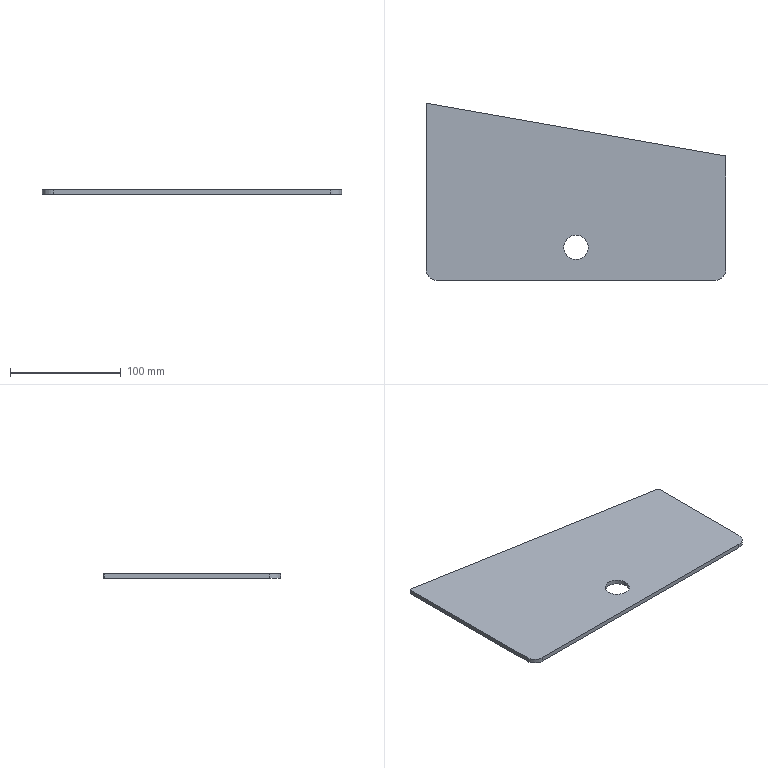Part | STEP file | 001-011-Blanking flip adjusting plate | 1 solid | 12 faces | box 270 x 159.808 x 4 mm | volume 145397 mm3 | cylinder 6 | plane 6 | commonest cylinder face diameters 2 x2 20 x2 22 x2
STEP:
#1=CARTESIAN_POINT('',(0.,0.,0.));
#2=DIRECTION('',(0.,0.,1.));
#3=DIRECTION('',(1.,0.,0.));
#4=AXIS2_PLACEMENT_3D('',#1,#2,#3);
#5=CARTESIAN_POINT('',(-11.,-50.,0.));
#6=VERTEX_POINT('',#5);
#7=CARTESIAN_POINT('',(-11.,-50.,-4.));
#8=VERTEX_POINT('',#7);
#9=CARTESIAN_POINT('',(-11.,-50.,-4.));
#10=DIRECTION('',(0.,0.,-1.));
#11=VECTOR('',#10,1.);
#12=LINE('',#9,#11);
#13=CARTESIAN_POINT('',(0.,-50.,-4.));
#14=DIRECTION('',(0.,0.,-1.));
#15=DIRECTION('',(-1.,0.,0.));
#16=AXIS2_PLACEMENT_3D('',#13,#14,#15);
#17=CYLINDRICAL_SURFACE('',#16,11.);
#18=CARTESIAN_POINT('',(6.283,0.));
#19=DIRECTION('',(0.,1.));
#20=VECTOR('',#19,1.);
#21=LINE('',#18,#20);
#22=(GEOMETRIC_REPRESENTATION_CONTEXT(2)PARAMETRIC_REPRESENTATION_CONTEXT()REPRESENTATION_CONTEXT('',''));
#23=DEFINITIONAL_REPRESENTATION('',(#21),#22);
#24=PCURVE('',#17,#23);
#25=CARTESIAN_POINT('',(0.,-50.,-4.));
#26=DIRECTION('',(0.,0.,-1.));
#27=DIRECTION('',(-1.,0.,0.));
#28=AXIS2_PLACEMENT_3D('',#25,#26,#27);
#29=CYLINDRICAL_SURFACE('',#28,11.);
#30=CARTESIAN_POINT('',(0.,0.));
#31=DIRECTION('',(0.,1.));
#32=VECTOR('',#31,1.);
#33=LINE('',#30,#32);
#34=(GEOMETRIC_REPRESENTATION_CONTEXT(2)PARAMETRIC_REPRESENTATION_CONTEXT()REPRESENTATION_CONTEXT('',''));
#35=DEFINITIONAL_REPRESENTATION('',(#33),#34);
#36=PCURVE('',#29,#35);
#37=SURFACE_CURVE('',#12,(#24,#36),.PCURVE_S1.);
#38=EDGE_CURVE('',#6,#8,#37,.T.);
#39=ORIENTED_EDGE('',*,*,#38,.T.);
#40=CARTESIAN_POINT('',(11.,-50.,-4.));
#41=VERTEX_POINT('',#40);
#42=CARTESIAN_POINT('',(0.,-50.,-4.));
#43=DIRECTION('',(0.,0.,-1.));
#44=DIRECTION('',(-1.,0.,0.));
#45=AXIS2_PLACEMENT_3D('',#42,#43,#44);
#46=CIRCLE('',#45,11.);
#47=CARTESIAN_POINT('',(0.,0.));
#48=DIRECTION('',(1.,0.));
#49=VECTOR('',#48,1.);
#50=LINE('',#47,#49);
#51=(GEOMETRIC_REPRESENTATION_CONTEXT(2)PARAMETRIC_REPRESENTATION_CONTEXT()REPRESENTATION_CONTEXT('',''));
#52=DEFINITIONAL_REPRESENTATION('',(#50),#51);
#53=PCURVE('',#17,#52);
#54=CARTESIAN_POINT('',(0.,0.,-4.));
#55=DIRECTION('',(0.,0.,-1.));
#56=DIRECTION('',(-1.,0.,0.));
#57=AXIS2_PLACEMENT_3D('',#54,#55,#56);
#58=PLANE('',#57);
#59=CARTESIAN_POINT('',(0.,-50.));
#60=DIRECTION('',(1.,0.));
#61=AXIS2_PLACEMENT_2D('',#59,#60);
#62=CIRCLE('',#61,11.);
#63=(GEOMETRIC_REPRESENTATION_CONTEXT(2)PARAMETRIC_REPRESENTATION_CONTEXT()REPRESENTATION_CONTEXT('',''));
#64=DEFINITIONAL_REPRESENTATION('',(#62),#63);
#65=PCURVE('',#58,#64);
#66=SURFACE_CURVE('',#46,(#53,#65),.PCURVE_S1.);
#67=EDGE_CURVE('',#41,#8,#66,.T.);
#68=ORIENTED_EDGE('',*,*,#67,.F.);
#69=CARTESIAN_POINT('',(11.,-50.,0.));
#70=VERTEX_POINT('',#69);
#71=CARTESIAN_POINT('',(11.,-50.,-4.));
#72=DIRECTION('',(0.,0.,-1.));
#73=VECTOR('',#72,1.);
#74=LINE('',#71,#73);
#75=CARTESIAN_POINT('',(3.142,0.));
#76=DIRECTION('',(0.,1.));
#77=VECTOR('',#76,1.);
#78=LINE('',#75,#77);
#79=(GEOMETRIC_REPRESENTATION_CONTEXT(2)PARAMETRIC_REPRESENTATION_CONTEXT()REPRESENTATION_CONTEXT('',''));
#80=DEFINITIONAL_REPRESENTATION('',(#78),#79);
#81=PCURVE('',#17,#80);
#82=CARTESIAN_POINT('',(3.142,0.));
#83=DIRECTION('',(0.,1.));
#84=VECTOR('',#83,1.);
#85=LINE('',#82,#84);
#86=(GEOMETRIC_REPRESENTATION_CONTEXT(2)PARAMETRIC_REPRESENTATION_CONTEXT()REPRESENTATION_CONTEXT('',''));
#87=DEFINITIONAL_REPRESENTATION('',(#85),#86);
#88=PCURVE('',#29,#87);
#89=SURFACE_CURVE('',#74,(#81,#88),.PCURVE_S1.);
#90=EDGE_CURVE('',#70,#41,#89,.T.);
#91=ORIENTED_EDGE('',*,*,#90,.F.);
#92=CARTESIAN_POINT('',(0.,-50.,0.));
#93=DIRECTION('',(0.,0.,-1.));
#94=DIRECTION('',(-1.,0.,0.));
#95=AXIS2_PLACEMENT_3D('',#92,#93,#94);
#96=CIRCLE('',#95,11.);
#97=CARTESIAN_POINT('',(0.,-4.));
#98=DIRECTION('',(1.,0.));
#99=VECTOR('',#98,1.);
#100=LINE('',#97,#99);
#101=(GEOMETRIC_REPRESENTATION_CONTEXT(2)PARAMETRIC_REPRESENTATION_CONTEXT()REPRESENTATION_CONTEXT('',''));
#102=DEFINITIONAL_REPRESENTATION('',(#100),#101);
#103=PCURVE('',#17,#102);
#104=CARTESIAN_POINT('',(0.,0.,0.));
#105=DIRECTION('',(0.,0.,-1.));
#106=DIRECTION('',(-1.,0.,0.));
#107=AXIS2_PLACEMENT_3D('',#104,#105,#106);
#108=PLANE('',#107);
#109=CARTESIAN_POINT('',(0.,-50.));
#110=DIRECTION('',(1.,0.));
#111=AXIS2_PLACEMENT_2D('',#109,#110);
#112=CIRCLE('',#111,11.);
#113=(GEOMETRIC_REPRESENTATION_CONTEXT(2)PARAMETRIC_REPRESENTATION_CONTEXT()REPRESENTATION_CONTEXT('',''));
#114=DEFINITIONAL_REPRESENTATION('',(#112),#113);
#115=PCURVE('',#108,#114);
#116=SURFACE_CURVE('',#96,(#103,#115),.PCURVE_S1.);
#117=EDGE_CURVE('',#70,#6,#116,.T.);
#118=ORIENTED_EDGE('',*,*,#117,.T.);
#119=EDGE_LOOP('',(#39,#68,#91,#118));
#120=FACE_BOUND('',#119,.F.);
#121=ADVANCED_FACE('',(#120),#17,.F.);
#122=CARTESIAN_POINT('',(135.,-70.,-4.));
#123=VERTEX_POINT('',#122);
#124=CARTESIAN_POINT('',(135.,31.553,-4.));
#125=VERTEX_POINT('',#124);
#126=CARTESIAN_POINT('',(135.,-80.,-4.));
#127=DIRECTION('',(0.,1.,0.));
#128=VECTOR('',#127,1.);
#129=LINE('',#126,#128);
#130=CARTESIAN_POINT('',(135.,-80.,-4.));
#131=DIRECTION('',(1.,0.,0.));
#132=DIRECTION('',(0.,1.,0.));
#133=AXIS2_PLACEMENT_3D('',#130,#131,#132);
#134=PLANE('',#133);
#135=CARTESIAN_POINT('',(0.,0.));
#136=DIRECTION('',(1.,0.));
#137=VECTOR('',#136,1.);
#138=LINE('',#135,#137);
#139=(GEOMETRIC_REPRESENTATION_CONTEXT(2)PARAMETRIC_REPRESENTATION_CONTEXT()REPRESENTATION_CONTEXT('',''));
#140=DEFINITIONAL_REPRESENTATION('',(#138),#139);
#141=PCURVE('',#134,#140);
#142=CARTESIAN_POINT('',(-135.,-80.));
#143=DIRECTION('',(0.,1.));
#144=VECTOR('',#143,1.);
#145=LINE('',#142,#144);
#146=(GEOMETRIC_REPRESENTATION_CONTEXT(2)PARAMETRIC_REPRESENTATION_CONTEXT()REPRESENTATION_CONTEXT('',''));
#147=DEFINITIONAL_REPRESENTATION('',(#145),#146);
#148=PCURVE('',#58,#147);
#149=SURFACE_CURVE('',#129,(#141,#148),.PCURVE_S1.);
#150=EDGE_CURVE('',#123,#125,#149,.T.);
#151=ORIENTED_EDGE('',*,*,#150,.T.);
#152=CARTESIAN_POINT('',(135.,31.553,0.));
#153=VERTEX_POINT('',#152);
#154=CARTESIAN_POINT('',(135.,31.553,0.));
#155=DIRECTION('',(0.,0.,1.));
#156=VECTOR('',#155,1.);
#157=LINE('',#154,#156);
#158=CARTESIAN_POINT('',(111.553,4.));
#159=DIRECTION('',(0.,1.));
#160=VECTOR('',#159,1.);
#161=LINE('',#158,#160);
#162=(GEOMETRIC_REPRESENTATION_CONTEXT(2)PARAMETRIC_REPRESENTATION_CONTEXT()REPRESENTATION_CONTEXT('',''));
#163=DEFINITIONAL_REPRESENTATION('',(#161),#162);
#164=PCURVE('',#134,#163);
#165=CARTESIAN_POINT('',(134.,31.553,-4.));
#166=DIRECTION('',(0.,0.,-1.));
#167=DIRECTION('',(-1.,0.,0.));
#168=AXIS2_PLACEMENT_3D('',#165,#166,#167);
#169=CYLINDRICAL_SURFACE('',#168,1.);
#170=CARTESIAN_POINT('',(3.142,-4.));
#171=DIRECTION('',(0.,-1.));
#172=VECTOR('',#171,1.);
#173=LINE('',#170,#172);
#174=(GEOMETRIC_REPRESENTATION_CONTEXT(2)PARAMETRIC_REPRESENTATION_CONTEXT()REPRESENTATION_CONTEXT('',''));
#175=DEFINITIONAL_REPRESENTATION('',(#173),#174);
#176=PCURVE('',#169,#175);
#177=SURFACE_CURVE('',#157,(#164,#176),.PCURVE_S1.);
#178=EDGE_CURVE('',#125,#153,#177,.T.);
#179=ORIENTED_EDGE('',*,*,#178,.T.);
#180=CARTESIAN_POINT('',(135.,-70.,0.));
#181=VERTEX_POINT('',#180);
#182=CARTESIAN_POINT('',(135.,-80.,0.));
#183=DIRECTION('',(0.,1.,0.));
#184=VECTOR('',#183,1.);
#185=LINE('',#182,#184);
#186=CARTESIAN_POINT('',(0.,4.));
#187=DIRECTION('',(1.,0.));
#188=VECTOR('',#187,1.);
#189=LINE('',#186,#188);
#190=(GEOMETRIC_REPRESENTATION_CONTEXT(2)PARAMETRIC_REPRESENTATION_CONTEXT()REPRESENTATION_CONTEXT('',''));
#191=DEFINITIONAL_REPRESENTATION('',(#189),#190);
#192=PCURVE('',#134,#191);
#193=CARTESIAN_POINT('',(-135.,-80.));
#194=DIRECTION('',(0.,1.));
#195=VECTOR('',#194,1.);
#196=LINE('',#193,#195);
#197=(GEOMETRIC_REPRESENTATION_CONTEXT(2)PARAMETRIC_REPRESENTATION_CONTEXT()REPRESENTATION_CONTEXT('',''));
#198=DEFINITIONAL_REPRESENTATION('',(#196),#197);
#199=PCURVE('',#108,#198);
#200=SURFACE_CURVE('',#185,(#192,#199),.PCURVE_S1.);
#201=EDGE_CURVE('',#181,#153,#200,.T.);
#202=ORIENTED_EDGE('',*,*,#201,.F.);
#203=CARTESIAN_POINT('',(135.,-70.,-4.));
#204=DIRECTION('',(0.,0.,-1.));
#205=VECTOR('',#204,1.);
#206=LINE('',#203,#205);
#207=CARTESIAN_POINT('',(10.,0.));
#208=DIRECTION('',(0.,-1.));
#209=VECTOR('',#208,1.);
#210=LINE('',#207,#209);
#211=(GEOMETRIC_REPRESENTATION_CONTEXT(2)PARAMETRIC_REPRESENTATION_CONTEXT()REPRESENTATION_CONTEXT('',''));
#212=DEFINITIONAL_REPRESENTATION('',(#210),#211);
#213=PCURVE('',#134,#212);
#214=CARTESIAN_POINT('',(125.,-70.,-4.));
#215=DIRECTION('',(0.,0.,1.));
#216=DIRECTION('',(1.,0.,0.));
#217=AXIS2_PLACEMENT_3D('',#214,#215,#216);
#218=CYLINDRICAL_SURFACE('',#217,10.);
#219=CARTESIAN_POINT('',(6.283,0.));
#220=DIRECTION('',(0.,-1.));
#221=VECTOR('',#220,1.);
#222=LINE('',#219,#221);
#223=(GEOMETRIC_REPRESENTATION_CONTEXT(2)PARAMETRIC_REPRESENTATION_CONTEXT()REPRESENTATION_CONTEXT('',''));
#224=DEFINITIONAL_REPRESENTATION('',(#222),#223);
#225=PCURVE('',#218,#224);
#226=SURFACE_CURVE('',#206,(#213,#225),.PCURVE_S1.);
#227=EDGE_CURVE('',#181,#123,#226,.T.);
#228=ORIENTED_EDGE('',*,*,#227,.T.);
#229=EDGE_LOOP('',(#151,#179,#202,#228));
#230=FACE_BOUND('',#229,.T.);
#231=ADVANCED_FACE('',(#230),#134,.T.);
#232=CARTESIAN_POINT('',(-125.,-80.,0.));
#233=VERTEX_POINT('',#232);
#234=CARTESIAN_POINT('',(125.,-80.,0.));
#235=VERTEX_POINT('',#234);
#236=CARTESIAN_POINT('',(-135.,-80.,0.));
#237=DIRECTION('',(1.,0.,0.));
#238=VECTOR('',#237,1.);
#239=LINE('',#236,#238);
#240=CARTESIAN_POINT('',(-135.,-80.,-4.));
#241=DIRECTION('',(0.,-1.,0.));
#242=DIRECTION('',(0.,0.,-1.));
#243=AXIS2_PLACEMENT_3D('',#240,#241,#242);
#244=PLANE('',#243);
#245=CARTESIAN_POINT('',(-4.,0.));
#246=DIRECTION('',(0.,1.));
#247=VECTOR('',#246,1.);
#248=LINE('',#245,#247);
#249=(GEOMETRIC_REPRESENTATION_CONTEXT(2)PARAMETRIC_REPRESENTATION_CONTEXT()REPRESENTATION_CONTEXT('',''));
#250=DEFINITIONAL_REPRESENTATION('',(#248),#249);
#251=PCURVE('',#244,#250);
#252=CARTESIAN_POINT('',(135.,-80.));
#253=DIRECTION('',(-1.,0.));
#254=VECTOR('',#253,1.);
#255=LINE('',#252,#254);
#256=(GEOMETRIC_REPRESENTATION_CONTEXT(2)PARAMETRIC_REPRESENTATION_CONTEXT()REPRESENTATION_CONTEXT('',''));
#257=DEFINITIONAL_REPRESENTATION('',(#255),#256);
#258=PCURVE('',#108,#257);
#259=SURFACE_CURVE('',#239,(#251,#258),.PCURVE_S1.);
#260=EDGE_CURVE('',#233,#235,#259,.T.);
#261=ORIENTED_EDGE('',*,*,#260,.F.);
#262=CARTESIAN_POINT('',(-125.,-80.,-4.));
#263=VERTEX_POINT('',#262);
#264=CARTESIAN_POINT('',(-125.,-80.,-4.));
#265=DIRECTION('',(0.,0.,-1.));
#266=VECTOR('',#265,1.);
#267=LINE('',#264,#266);
#268=CARTESIAN_POINT('',(0.,10.));
#269=DIRECTION('',(1.,0.));
#270=VECTOR('',#269,1.);
#271=LINE('',#268,#270);
#272=(GEOMETRIC_REPRESENTATION_CONTEXT(2)PARAMETRIC_REPRESENTATION_CONTEXT()REPRESENTATION_CONTEXT('',''));
#273=DEFINITIONAL_REPRESENTATION('',(#271),#272);
#274=PCURVE('',#244,#273);
#275=CARTESIAN_POINT('',(-125.,-70.,-4.));
#276=DIRECTION('',(0.,0.,1.));
#277=DIRECTION('',(1.,0.,0.));
#278=AXIS2_PLACEMENT_3D('',#275,#276,#277);
#279=CYLINDRICAL_SURFACE('',#278,10.);
#280=CARTESIAN_POINT('',(4.712,0.));
#281=DIRECTION('',(0.,-1.));
#282=VECTOR('',#281,1.);
#283=LINE('',#280,#282);
#284=(GEOMETRIC_REPRESENTATION_CONTEXT(2)PARAMETRIC_REPRESENTATION_CONTEXT()REPRESENTATION_CONTEXT('',''));
#285=DEFINITIONAL_REPRESENTATION('',(#283),#284);
#286=PCURVE('',#279,#285);
#287=SURFACE_CURVE('',#267,(#274,#286),.PCURVE_S1.);
#288=EDGE_CURVE('',#233,#263,#287,.T.);
#289=ORIENTED_EDGE('',*,*,#288,.T.);
#290=CARTESIAN_POINT('',(125.,-80.,-4.));
#291=VERTEX_POINT('',#290);
#292=CARTESIAN_POINT('',(-135.,-80.,-4.));
#293=DIRECTION('',(1.,0.,0.));
#294=VECTOR('',#293,1.);
#295=LINE('',#292,#294);
#296=CARTESIAN_POINT('',(0.,0.));
#297=DIRECTION('',(0.,1.));
#298=VECTOR('',#297,1.);
#299=LINE('',#296,#298);
#300=(GEOMETRIC_REPRESENTATION_CONTEXT(2)PARAMETRIC_REPRESENTATION_CONTEXT()REPRESENTATION_CONTEXT('',''));
#301=DEFINITIONAL_REPRESENTATION('',(#299),#300);
#302=PCURVE('',#244,#301);
#303=CARTESIAN_POINT('',(135.,-80.));
#304=DIRECTION('',(-1.,0.));
#305=VECTOR('',#304,1.);
#306=LINE('',#303,#305);
#307=(GEOMETRIC_REPRESENTATION_CONTEXT(2)PARAMETRIC_REPRESENTATION_CONTEXT()REPRESENTATION_CONTEXT('',''));
#308=DEFINITIONAL_REPRESENTATION('',(#306),#307);
#309=PCURVE('',#58,#308);
#310=SURFACE_CURVE('',#295,(#302,#309),.PCURVE_S1.);
#311=EDGE_CURVE('',#263,#291,#310,.T.);
#312=ORIENTED_EDGE('',*,*,#311,.T.);
#313=CARTESIAN_POINT('',(125.,-80.,-4.));
#314=DIRECTION('',(0.,0.,1.));
#315=VECTOR('',#314,1.);
#316=LINE('',#313,#315);
#317=CARTESIAN_POINT('',(0.,260.));
#318=DIRECTION('',(-1.,0.));
#319=VECTOR('',#318,1.);
#320=LINE('',#317,#319);
#321=(GEOMETRIC_REPRESENTATION_CONTEXT(2)PARAMETRIC_REPRESENTATION_CONTEXT()REPRESENTATION_CONTEXT('',''));
#322=DEFINITIONAL_REPRESENTATION('',(#320),#321);
#323=PCURVE('',#244,#322);
#324=CARTESIAN_POINT('',(4.712,0.));
#325=DIRECTION('',(0.,1.));
#326=VECTOR('',#325,1.);
#327=LINE('',#324,#326);
#328=(GEOMETRIC_REPRESENTATION_CONTEXT(2)PARAMETRIC_REPRESENTATION_CONTEXT()REPRESENTATION_CONTEXT('',''));
#329=DEFINITIONAL_REPRESENTATION('',(#327),#328);
#330=PCURVE('',#218,#329);
#331=SURFACE_CURVE('',#316,(#323,#330),.PCURVE_S1.);
#332=EDGE_CURVE('',#291,#235,#331,.T.);
#333=ORIENTED_EDGE('',*,*,#332,.T.);
#334=EDGE_LOOP('',(#261,#289,#312,#333));
#335=FACE_BOUND('',#334,.T.);
#336=ADVANCED_FACE('',(#335),#244,.T.);
#337=CARTESIAN_POINT('',(-135.,78.808,0.));
#338=VERTEX_POINT('',#337);
#339=CARTESIAN_POINT('',(-135.,-70.,0.));
#340=VERTEX_POINT('',#339);
#341=CARTESIAN_POINT('',(-135.,-80.,0.));
#342=DIRECTION('',(0.,-1.,0.));
#343=VECTOR('',#342,1.);
#344=LINE('',#341,#343);
#345=CARTESIAN_POINT('',(-135.,-80.,-4.));
#346=DIRECTION('',(-1.,0.,0.));
#347=DIRECTION('',(0.,-1.,0.));
#348=AXIS2_PLACEMENT_3D('',#345,#346,#347);
#349=PLANE('',#348);
#350=CARTESIAN_POINT('',(0.,4.));
#351=DIRECTION('',(1.,0.));
#352=VECTOR('',#351,1.);
#353=LINE('',#350,#352);
#354=(GEOMETRIC_REPRESENTATION_CONTEXT(2)PARAMETRIC_REPRESENTATION_CONTEXT()REPRESENTATION_CONTEXT('',''));
#355=DEFINITIONAL_REPRESENTATION('',(#353),#354);
#356=PCURVE('',#349,#355);
#357=CARTESIAN_POINT('',(135.,-80.));
#358=DIRECTION('',(0.,-1.));
#359=VECTOR('',#358,1.);
#360=LINE('',#357,#359);
#361=(GEOMETRIC_REPRESENTATION_CONTEXT(2)PARAMETRIC_REPRESENTATION_CONTEXT()REPRESENTATION_CONTEXT('',''));
#362=DEFINITIONAL_REPRESENTATION('',(#360),#361);
#363=PCURVE('',#108,#362);
#364=SURFACE_CURVE('',#344,(#356,#363),.PCURVE_S1.);
#365=EDGE_CURVE('',#338,#340,#364,.T.);
#366=ORIENTED_EDGE('',*,*,#365,.F.);
#367=CARTESIAN_POINT('',(-135.,78.808,-4.));
#368=VERTEX_POINT('',#367);
#369=CARTESIAN_POINT('',(-135.,78.808,-4.));
#370=DIRECTION('',(0.,0.,-1.));
#371=VECTOR('',#370,1.);
#372=LINE('',#369,#371);
#373=CARTESIAN_POINT('',(-158.808,0.));
#374=DIRECTION('',(0.,-1.));
#375=VECTOR('',#374,1.);
#376=LINE('',#373,#375);
#377=(GEOMETRIC_REPRESENTATION_CONTEXT(2)PARAMETRIC_REPRESENTATION_CONTEXT()REPRESENTATION_CONTEXT('',''));
#378=DEFINITIONAL_REPRESENTATION('',(#376),#377);
#379=PCURVE('',#349,#378);
#380=CARTESIAN_POINT('',(-134.,78.808,-4.));
#381=DIRECTION('',(0.,0.,-1.));
#382=DIRECTION('',(-1.,0.,0.));
#383=AXIS2_PLACEMENT_3D('',#380,#381,#382);
#384=CYLINDRICAL_SURFACE('',#383,1.);
#385=CARTESIAN_POINT('',(0.,0.));
#386=DIRECTION('',(0.,1.));
#387=VECTOR('',#386,1.);
#388=LINE('',#385,#387);
#389=(GEOMETRIC_REPRESENTATION_CONTEXT(2)PARAMETRIC_REPRESENTATION_CONTEXT()REPRESENTATION_CONTEXT('',''));
#390=DEFINITIONAL_REPRESENTATION('',(#388),#389);
#391=PCURVE('',#384,#390);
#392=SURFACE_CURVE('',#372,(#379,#391),.PCURVE_S1.);
#393=EDGE_CURVE('',#338,#368,#392,.T.);
#394=ORIENTED_EDGE('',*,*,#393,.T.);
#395=CARTESIAN_POINT('',(-135.,-70.,-4.));
#396=VERTEX_POINT('',#395);
#397=CARTESIAN_POINT('',(-135.,-80.,-4.));
#398=DIRECTION('',(0.,-1.,0.));
#399=VECTOR('',#398,1.);
#400=LINE('',#397,#399);
#401=CARTESIAN_POINT('',(0.,0.));
#402=DIRECTION('',(1.,0.));
#403=VECTOR('',#402,1.);
#404=LINE('',#401,#403);
#405=(GEOMETRIC_REPRESENTATION_CONTEXT(2)PARAMETRIC_REPRESENTATION_CONTEXT()REPRESENTATION_CONTEXT('',''));
#406=DEFINITIONAL_REPRESENTATION('',(#404),#405);
#407=PCURVE('',#349,#406);
#408=CARTESIAN_POINT('',(135.,-80.));
#409=DIRECTION('',(0.,-1.));
#410=VECTOR('',#409,1.);
#411=LINE('',#408,#410);
#412=(GEOMETRIC_REPRESENTATION_CONTEXT(2)PARAMETRIC_REPRESENTATION_CONTEXT()REPRESENTATION_CONTEXT('',''));
#413=DEFINITIONAL_REPRESENTATION('',(#411),#412);
#414=PCURVE('',#58,#413);
#415=SURFACE_CURVE('',#400,(#407,#414),.PCURVE_S1.);
#416=EDGE_CURVE('',#368,#396,#415,.T.);
#417=ORIENTED_EDGE('',*,*,#416,.T.);
#418=CARTESIAN_POINT('',(-135.,-70.,-4.));
#419=DIRECTION('',(0.,0.,1.));
#420=VECTOR('',#419,1.);
#421=LINE('',#418,#420);
#422=CARTESIAN_POINT('',(-10.,0.));
#423=DIRECTION('',(0.,1.));
#424=VECTOR('',#423,1.);
#425=LINE('',#422,#424);
#426=(GEOMETRIC_REPRESENTATION_CONTEXT(2)PARAMETRIC_REPRESENTATION_CONTEXT()REPRESENTATION_CONTEXT('',''));
#427=DEFINITIONAL_REPRESENTATION('',(#425),#426);
#428=PCURVE('',#349,#427);
#429=CARTESIAN_POINT('',(3.142,0.));
#430=DIRECTION('',(0.,1.));
#431=VECTOR('',#430,1.);
#432=LINE('',#429,#431);
#433=(GEOMETRIC_REPRESENTATION_CONTEXT(2)PARAMETRIC_REPRESENTATION_CONTEXT()REPRESENTATION_CONTEXT('',''));
#434=DEFINITIONAL_REPRESENTATION('',(#432),#433);
#435=PCURVE('',#279,#434);
#436=SURFACE_CURVE('',#421,(#428,#435),.PCURVE_S1.);
#437=EDGE_CURVE('',#396,#340,#436,.T.);
#438=ORIENTED_EDGE('',*,*,#437,.T.);
#439=EDGE_LOOP('',(#366,#394,#417,#438));
#440=FACE_BOUND('',#439,.T.);
#441=ADVANCED_FACE('',(#440),#349,.T.);
#442=CARTESIAN_POINT('',(0.,-50.,-4.));
#443=DIRECTION('',(0.,0.,-1.));
#444=DIRECTION('',(-1.,0.,0.));
#445=AXIS2_PLACEMENT_3D('',#442,#443,#444);
#446=CIRCLE('',#445,11.);
#447=CARTESIAN_POINT('',(0.,-50.));
#448=DIRECTION('',(1.,0.));
#449=AXIS2_PLACEMENT_2D('',#447,#448);
#450=CIRCLE('',#449,11.);
#451=(GEOMETRIC_REPRESENTATION_CONTEXT(2)PARAMETRIC_REPRESENTATION_CONTEXT()REPRESENTATION_CONTEXT('',''));
#452=DEFINITIONAL_REPRESENTATION('',(#450),#451);
#453=PCURVE('',#58,#452);
#454=CARTESIAN_POINT('',(0.,0.));
#455=DIRECTION('',(1.,0.));
#456=VECTOR('',#455,1.);
#457=LINE('',#454,#456);
#458=(GEOMETRIC_REPRESENTATION_CONTEXT(2)PARAMETRIC_REPRESENTATION_CONTEXT()REPRESENTATION_CONTEXT('',''));
#459=DEFINITIONAL_REPRESENTATION('',(#457),#458);
#460=PCURVE('',#29,#459);
#461=SURFACE_CURVE('',#446,(#453,#460),.PCURVE_S1.);
#462=EDGE_CURVE('',#8,#41,#461,.T.);
#463=ORIENTED_EDGE('',*,*,#462,.F.);
#464=ORIENTED_EDGE('',*,*,#67,.F.);
#465=EDGE_LOOP('',(#463,#464));
#466=FACE_BOUND('',#465,.T.);
#467=ORIENTED_EDGE('',*,*,#416,.F.);
#468=CARTESIAN_POINT('',(-133.826,79.793,-4.));
#469=VERTEX_POINT('',#468);
#470=CARTESIAN_POINT('',(-134.,78.808,-4.));
#471=DIRECTION('',(0.,0.,-1.));
#472=DIRECTION('',(-1.,0.,0.));
#473=AXIS2_PLACEMENT_3D('',#470,#471,#472);
#474=CIRCLE('',#473,1.);
#475=CARTESIAN_POINT('',(134.,78.808));
#476=DIRECTION('',(1.,0.));
#477=AXIS2_PLACEMENT_2D('',#475,#476);
#478=CIRCLE('',#477,1.);
#479=(GEOMETRIC_REPRESENTATION_CONTEXT(2)PARAMETRIC_REPRESENTATION_CONTEXT()REPRESENTATION_CONTEXT('',''));
#480=DEFINITIONAL_REPRESENTATION('',(#478),#479);
#481=PCURVE('',#58,#480);
#482=CARTESIAN_POINT('',(0.,0.));
#483=DIRECTION('',(1.,0.));
#484=VECTOR('',#483,1.);
#485=LINE('',#482,#484);
#486=(GEOMETRIC_REPRESENTATION_CONTEXT(2)PARAMETRIC_REPRESENTATION_CONTEXT()REPRESENTATION_CONTEXT('',''));
#487=DEFINITIONAL_REPRESENTATION('',(#485),#486);
#488=PCURVE('',#384,#487);
#489=SURFACE_CURVE('',#474,(#481,#488),.PCURVE_S1.);
#490=EDGE_CURVE('',#368,#469,#489,.T.);
#491=ORIENTED_EDGE('',*,*,#490,.T.);
#492=CARTESIAN_POINT('',(134.174,32.537,-4.));
#493=VERTEX_POINT('',#492);
#494=CARTESIAN_POINT('',(135.,32.392,-4.));
#495=DIRECTION('',(0.9848,-0.1736,0.));
#496=VECTOR('',#495,1.);
#497=LINE('',#494,#496);
#498=CARTESIAN_POINT('',(-135.,32.392));
#499=DIRECTION('',(-0.9848,-0.1736));
#500=VECTOR('',#499,1.);
#501=LINE('',#498,#500);
#502=(GEOMETRIC_REPRESENTATION_CONTEXT(2)PARAMETRIC_REPRESENTATION_CONTEXT()REPRESENTATION_CONTEXT('',''));
#503=DEFINITIONAL_REPRESENTATION('',(#501),#502);
#504=PCURVE('',#58,#503);
#505=CARTESIAN_POINT('',(135.,32.392,-4.));
#506=DIRECTION('',(-0.1736,-0.9848,0.));
#507=DIRECTION('',(0.9848,-0.1736,0.));
#508=AXIS2_PLACEMENT_3D('',#505,#506,#507);
#509=PLANE('',#508);
#510=CARTESIAN_POINT('',(0.,0.));
#511=DIRECTION('',(1.,0.));
#512=VECTOR('',#511,1.);
#513=LINE('',#510,#512);
#514=(GEOMETRIC_REPRESENTATION_CONTEXT(2)PARAMETRIC_REPRESENTATION_CONTEXT()REPRESENTATION_CONTEXT('',''));
#515=DEFINITIONAL_REPRESENTATION('',(#513),#514);
#516=PCURVE('',#509,#515);
#517=SURFACE_CURVE('',#497,(#504,#516),.PCURVE_S1.);
#518=EDGE_CURVE('',#469,#493,#517,.T.);
#519=ORIENTED_EDGE('',*,*,#518,.T.);
#520=CARTESIAN_POINT('',(134.,31.553,-4.));
#521=DIRECTION('',(0.,0.,-1.));
#522=DIRECTION('',(-1.,0.,0.));
#523=AXIS2_PLACEMENT_3D('',#520,#521,#522);
#524=CIRCLE('',#523,1.);
#525=CARTESIAN_POINT('',(-134.,31.553));
#526=DIRECTION('',(1.,0.));
#527=AXIS2_PLACEMENT_2D('',#525,#526);
#528=CIRCLE('',#527,1.);
#529=(GEOMETRIC_REPRESENTATION_CONTEXT(2)PARAMETRIC_REPRESENTATION_CONTEXT()REPRESENTATION_CONTEXT('',''));
#530=DEFINITIONAL_REPRESENTATION('',(#528),#529);
#531=PCURVE('',#58,#530);
#532=CARTESIAN_POINT('',(0.,0.));
#533=DIRECTION('',(1.,0.));
#534=VECTOR('',#533,1.);
#535=LINE('',#532,#534);
#536=(GEOMETRIC_REPRESENTATION_CONTEXT(2)PARAMETRIC_REPRESENTATION_CONTEXT()REPRESENTATION_CONTEXT('',''));
#537=DEFINITIONAL_REPRESENTATION('',(#535),#536);
#538=PCURVE('',#169,#537);
#539=SURFACE_CURVE('',#524,(#531,#538),.PCURVE_S1.);
#540=EDGE_CURVE('',#493,#125,#539,.T.);
#541=ORIENTED_EDGE('',*,*,#540,.T.);
#542=ORIENTED_EDGE('',*,*,#150,.F.);
#543=CARTESIAN_POINT('',(125.,-70.,-4.));
#544=DIRECTION('',(0.,0.,-1.));
#545=DIRECTION('',(-1.,0.,0.));
#546=AXIS2_PLACEMENT_3D('',#543,#544,#545);
#547=CIRCLE('',#546,10.);
#548=CARTESIAN_POINT('',(-125.,-70.));
#549=DIRECTION('',(1.,0.));
#550=AXIS2_PLACEMENT_2D('',#548,#549);
#551=CIRCLE('',#550,10.);
#552=(GEOMETRIC_REPRESENTATION_CONTEXT(2)PARAMETRIC_REPRESENTATION_CONTEXT()REPRESENTATION_CONTEXT('',''));
#553=DEFINITIONAL_REPRESENTATION('',(#551),#552);
#554=PCURVE('',#58,#553);
#555=CARTESIAN_POINT('',(9.425,0.));
#556=DIRECTION('',(-1.,0.));
#557=VECTOR('',#556,1.);
#558=LINE('',#555,#557);
#559=(GEOMETRIC_REPRESENTATION_CONTEXT(2)PARAMETRIC_REPRESENTATION_CONTEXT()REPRESENTATION_CONTEXT('',''));
#560=DEFINITIONAL_REPRESENTATION('',(#558),#559);
#561=PCURVE('',#218,#560);
#562=SURFACE_CURVE('',#547,(#554,#561),.PCURVE_S1.);
#563=EDGE_CURVE('',#123,#291,#562,.T.);
#564=ORIENTED_EDGE('',*,*,#563,.T.);
#565=ORIENTED_EDGE('',*,*,#311,.F.);
#566=CARTESIAN_POINT('',(-125.,-70.,-4.));
#567=DIRECTION('',(0.,0.,-1.));
#568=DIRECTION('',(-1.,0.,0.));
#569=AXIS2_PLACEMENT_3D('',#566,#567,#568);
#570=CIRCLE('',#569,10.);
#571=CARTESIAN_POINT('',(125.,-70.));
#572=DIRECTION('',(1.,0.));
#573=AXIS2_PLACEMENT_2D('',#571,#572);
#574=CIRCLE('',#573,10.);
#575=(GEOMETRIC_REPRESENTATION_CONTEXT(2)PARAMETRIC_REPRESENTATION_CONTEXT()REPRESENTATION_CONTEXT('',''));
#576=DEFINITIONAL_REPRESENTATION('',(#574),#575);
#577=PCURVE('',#58,#576);
#578=CARTESIAN_POINT('',(9.425,0.));
#579=DIRECTION('',(-1.,0.));
#580=VECTOR('',#579,1.);
#581=LINE('',#578,#580);
#582=(GEOMETRIC_REPRESENTATION_CONTEXT(2)PARAMETRIC_REPRESENTATION_CONTEXT()REPRESENTATION_CONTEXT('',''));
#583=DEFINITIONAL_REPRESENTATION('',(#581),#582);
#584=PCURVE('',#279,#583);
#585=SURFACE_CURVE('',#570,(#577,#584),.PCURVE_S1.);
#586=EDGE_CURVE('',#263,#396,#585,.T.);
#587=ORIENTED_EDGE('',*,*,#586,.T.);
#588=EDGE_LOOP('',(#467,#491,#519,#541,#542,#564,#565,#587));
#589=FACE_BOUND('',#588,.T.);
#590=ADVANCED_FACE('',(#466,#589),#58,.T.);
#591=CARTESIAN_POINT('',(0.,-50.,0.));
#592=DIRECTION('',(0.,0.,-1.));
#593=DIRECTION('',(-1.,0.,0.));
#594=AXIS2_PLACEMENT_3D('',#591,#592,#593);
#595=CIRCLE('',#594,11.);
#596=CARTESIAN_POINT('',(0.,-50.));
#597=DIRECTION('',(1.,0.));
#598=AXIS2_PLACEMENT_2D('',#596,#597);
#599=CIRCLE('',#598,11.);
#600=(GEOMETRIC_REPRESENTATION_CONTEXT(2)PARAMETRIC_REPRESENTATION_CONTEXT()REPRESENTATION_CONTEXT('',''));
#601=DEFINITIONAL_REPRESENTATION('',(#599),#600);
#602=PCURVE('',#108,#601);
#603=CARTESIAN_POINT('',(0.,-4.));
#604=DIRECTION('',(1.,0.));
#605=VECTOR('',#604,1.);
#606=LINE('',#603,#605);
#607=(GEOMETRIC_REPRESENTATION_CONTEXT(2)PARAMETRIC_REPRESENTATION_CONTEXT()REPRESENTATION_CONTEXT('',''));
#608=DEFINITIONAL_REPRESENTATION('',(#606),#607);
#609=PCURVE('',#29,#608);
#610=SURFACE_CURVE('',#595,(#602,#609),.PCURVE_S1.);
#611=EDGE_CURVE('',#6,#70,#610,.T.);
#612=ORIENTED_EDGE('',*,*,#611,.T.);
#613=ORIENTED_EDGE('',*,*,#117,.T.);
#614=EDGE_LOOP('',(#612,#613));
#615=FACE_BOUND('',#614,.T.);
#616=CARTESIAN_POINT('',(-133.826,79.793,0.));
#617=VERTEX_POINT('',#616);
#618=CARTESIAN_POINT('',(134.174,32.537,0.));
#619=VERTEX_POINT('',#618);
#620=CARTESIAN_POINT('',(135.,32.392,0.));
#621=DIRECTION('',(0.9848,-0.1736,0.));
#622=VECTOR('',#621,1.);
#623=LINE('',#620,#622);
#624=CARTESIAN_POINT('',(-135.,32.392));
#625=DIRECTION('',(-0.9848,-0.1736));
#626=VECTOR('',#625,1.);
#627=LINE('',#624,#626);
#628=(GEOMETRIC_REPRESENTATION_CONTEXT(2)PARAMETRIC_REPRESENTATION_CONTEXT()REPRESENTATION_CONTEXT('',''));
#629=DEFINITIONAL_REPRESENTATION('',(#627),#628);
#630=PCURVE('',#108,#629);
#631=CARTESIAN_POINT('',(0.,4.));
#632=DIRECTION('',(1.,0.));
#633=VECTOR('',#632,1.);
#634=LINE('',#631,#633);
#635=(GEOMETRIC_REPRESENTATION_CONTEXT(2)PARAMETRIC_REPRESENTATION_CONTEXT()REPRESENTATION_CONTEXT('',''));
#636=DEFINITIONAL_REPRESENTATION('',(#634),#635);
#637=PCURVE('',#509,#636);
#638=SURFACE_CURVE('',#623,(#630,#637),.PCURVE_S1.);
#639=EDGE_CURVE('',#617,#619,#638,.T.);
#640=ORIENTED_EDGE('',*,*,#639,.F.);
#641=CARTESIAN_POINT('',(-134.,78.808,0.));
#642=DIRECTION('',(0.,0.,1.));
#643=DIRECTION('',(-1.,0.,0.));
#644=AXIS2_PLACEMENT_3D('',#641,#642,#643);
#645=CIRCLE('',#644,1.);
#646=CARTESIAN_POINT('',(135.,78.808));
#647=CARTESIAN_POINT('',(135.,77.076));
#648=CARTESIAN_POINT('',(133.5,77.942));
#649=CARTESIAN_POINT('',(132.,78.808));
#650=CARTESIAN_POINT('',(133.5,79.674));
#651=CARTESIAN_POINT('',(135.,80.54));
#652=CARTESIAN_POINT('',(135.,78.808));
#653=(BOUNDED_CURVE()B_SPLINE_CURVE(2,(#646,#647,#648,#649,#650,#651,#652),.UNSPECIFIED.,.T.,.F.)B_SPLINE_CURVE_WITH_KNOTS((1,2,2,2,2,1),(-2.094,0.,2.094,4.189,6.283,8.378),.UNSPECIFIED.)CURVE()GEOMETRIC_REPRESENTATION_ITEM()RATIONAL_B_SPLINE_CURVE((1.,0.5,1.,0.5,1.,0.5,1.))REPRESENTATION_ITEM(''));
#654=(GEOMETRIC_REPRESENTATION_CONTEXT(2)PARAMETRIC_REPRESENTATION_CONTEXT()REPRESENTATION_CONTEXT('',''));
#655=DEFINITIONAL_REPRESENTATION('',(#653),#654);
#656=PCURVE('',#108,#655);
#657=CARTESIAN_POINT('',(6.283,-4.));
#658=DIRECTION('',(-1.,0.));
#659=VECTOR('',#658,1.);
#660=LINE('',#657,#659);
#661=(GEOMETRIC_REPRESENTATION_CONTEXT(2)PARAMETRIC_REPRESENTATION_CONTEXT()REPRESENTATION_CONTEXT('',''));
#662=DEFINITIONAL_REPRESENTATION('',(#660),#661);
#663=PCURVE('',#384,#662);
#664=SURFACE_CURVE('',#645,(#656,#663),.PCURVE_S1.);
#665=EDGE_CURVE('',#617,#338,#664,.T.);
#666=ORIENTED_EDGE('',*,*,#665,.T.);
#667=ORIENTED_EDGE('',*,*,#365,.T.);
#668=CARTESIAN_POINT('',(-125.,-70.,0.));
#669=DIRECTION('',(0.,0.,1.));
#670=DIRECTION('',(-1.,0.,0.));
#671=AXIS2_PLACEMENT_3D('',#668,#669,#670);
#672=CIRCLE('',#671,10.);
#673=CARTESIAN_POINT('',(135.,-70.));
#674=CARTESIAN_POINT('',(135.,-87.321));
#675=CARTESIAN_POINT('',(120.,-78.66));
#676=CARTESIAN_POINT('',(105.,-70.));
#677=CARTESIAN_POINT('',(120.,-61.34));
#678=CARTESIAN_POINT('',(135.,-52.679));
#679=CARTESIAN_POINT('',(135.,-70.));
#680=(BOUNDED_CURVE()B_SPLINE_CURVE(2,(#673,#674,#675,#676,#677,#678,#679),.UNSPECIFIED.,.T.,.F.)B_SPLINE_CURVE_WITH_KNOTS((1,2,2,2,2,1),(-2.094,0.,2.094,4.189,6.283,8.378),.UNSPECIFIED.)CURVE()GEOMETRIC_REPRESENTATION_ITEM()RATIONAL_B_SPLINE_CURVE((1.,0.5,1.,0.5,1.,0.5,1.))REPRESENTATION_ITEM(''));
#681=(GEOMETRIC_REPRESENTATION_CONTEXT(2)PARAMETRIC_REPRESENTATION_CONTEXT()REPRESENTATION_CONTEXT('',''));
#682=DEFINITIONAL_REPRESENTATION('',(#680),#681);
#683=PCURVE('',#108,#682);
#684=CARTESIAN_POINT('',(3.142,4.));
#685=DIRECTION('',(1.,0.));
#686=VECTOR('',#685,1.);
#687=LINE('',#684,#686);
#688=(GEOMETRIC_REPRESENTATION_CONTEXT(2)PARAMETRIC_REPRESENTATION_CONTEXT()REPRESENTATION_CONTEXT('',''));
#689=DEFINITIONAL_REPRESENTATION('',(#687),#688);
#690=PCURVE('',#279,#689);
#691=SURFACE_CURVE('',#672,(#683,#690),.PCURVE_S1.);
#692=EDGE_CURVE('',#340,#233,#691,.T.);
#693=ORIENTED_EDGE('',*,*,#692,.T.);
#694=ORIENTED_EDGE('',*,*,#260,.T.);
#695=CARTESIAN_POINT('',(125.,-70.,0.));
#696=DIRECTION('',(0.,0.,1.));
#697=DIRECTION('',(-1.,0.,0.));
#698=AXIS2_PLACEMENT_3D('',#695,#696,#697);
#699=CIRCLE('',#698,10.);
#700=CARTESIAN_POINT('',(-115.,-70.));
#701=CARTESIAN_POINT('',(-115.,-87.321));
#702=CARTESIAN_POINT('',(-130.,-78.66));
#703=CARTESIAN_POINT('',(-145.,-70.));
#704=CARTESIAN_POINT('',(-130.,-61.34));
#705=CARTESIAN_POINT('',(-115.,-52.679));
#706=CARTESIAN_POINT('',(-115.,-70.));
#707=(BOUNDED_CURVE()B_SPLINE_CURVE(2,(#700,#701,#702,#703,#704,#705,#706),.UNSPECIFIED.,.T.,.F.)B_SPLINE_CURVE_WITH_KNOTS((1,2,2,2,2,1),(-2.094,0.,2.094,4.189,6.283,8.378),.UNSPECIFIED.)CURVE()GEOMETRIC_REPRESENTATION_ITEM()RATIONAL_B_SPLINE_CURVE((1.,0.5,1.,0.5,1.,0.5,1.))REPRESENTATION_ITEM(''));
#708=(GEOMETRIC_REPRESENTATION_CONTEXT(2)PARAMETRIC_REPRESENTATION_CONTEXT()REPRESENTATION_CONTEXT('',''));
#709=DEFINITIONAL_REPRESENTATION('',(#707),#708);
#710=PCURVE('',#108,#709);
#711=CARTESIAN_POINT('',(3.142,4.));
#712=DIRECTION('',(1.,0.));
#713=VECTOR('',#712,1.);
#714=LINE('',#711,#713);
#715=(GEOMETRIC_REPRESENTATION_CONTEXT(2)PARAMETRIC_REPRESENTATION_CONTEXT()REPRESENTATION_CONTEXT('',''));
#716=DEFINITIONAL_REPRESENTATION('',(#714),#715);
#717=PCURVE('',#218,#716);
#718=SURFACE_CURVE('',#699,(#710,#717),.PCURVE_S1.);
#719=EDGE_CURVE('',#235,#181,#718,.T.);
#720=ORIENTED_EDGE('',*,*,#719,.T.);
#721=ORIENTED_EDGE('',*,*,#201,.T.);
#722=CARTESIAN_POINT('',(134.,31.553,0.));
#723=DIRECTION('',(0.,0.,1.));
#724=DIRECTION('',(-1.,0.,0.));
#725=AXIS2_PLACEMENT_3D('',#722,#723,#724);
#726=CIRCLE('',#725,1.);
#727=CARTESIAN_POINT('',(-133.,31.553));
#728=CARTESIAN_POINT('',(-133.,29.821));
#729=CARTESIAN_POINT('',(-134.5,30.687));
#730=CARTESIAN_POINT('',(-136.,31.553));
#731=CARTESIAN_POINT('',(-134.5,32.419));
#732=CARTESIAN_POINT('',(-133.,33.285));
#733=CARTESIAN_POINT('',(-133.,31.553));
#734=(BOUNDED_CURVE()B_SPLINE_CURVE(2,(#727,#728,#729,#730,#731,#732,#733),.UNSPECIFIED.,.T.,.F.)B_SPLINE_CURVE_WITH_KNOTS((1,2,2,2,2,1),(-2.094,0.,2.094,4.189,6.283,8.378),.UNSPECIFIED.)CURVE()GEOMETRIC_REPRESENTATION_ITEM()RATIONAL_B_SPLINE_CURVE((1.,0.5,1.,0.5,1.,0.5,1.))REPRESENTATION_ITEM(''));
#735=(GEOMETRIC_REPRESENTATION_CONTEXT(2)PARAMETRIC_REPRESENTATION_CONTEXT()REPRESENTATION_CONTEXT('',''));
#736=DEFINITIONAL_REPRESENTATION('',(#734),#735);
#737=PCURVE('',#108,#736);
#738=CARTESIAN_POINT('',(6.283,-4.));
#739=DIRECTION('',(-1.,0.));
#740=VECTOR('',#739,1.);
#741=LINE('',#738,#740);
#742=(GEOMETRIC_REPRESENTATION_CONTEXT(2)PARAMETRIC_REPRESENTATION_CONTEXT()REPRESENTATION_CONTEXT('',''));
#743=DEFINITIONAL_REPRESENTATION('',(#741),#742);
#744=PCURVE('',#169,#743);
#745=SURFACE_CURVE('',#726,(#737,#744),.PCURVE_S1.);
#746=EDGE_CURVE('',#153,#619,#745,.T.);
#747=ORIENTED_EDGE('',*,*,#746,.T.);
#748=EDGE_LOOP('',(#640,#666,#667,#693,#694,#720,#721,#747));
#749=FACE_BOUND('',#748,.T.);
#750=ADVANCED_FACE('',(#615,#749),#108,.F.);
#751=ORIENTED_EDGE('',*,*,#518,.F.);
#752=CARTESIAN_POINT('',(-133.826,79.793,0.));
#753=DIRECTION('',(0.,0.,1.));
#754=VECTOR('',#753,1.);
#755=LINE('',#752,#754);
#756=CARTESIAN_POINT('',(-272.973,4.));
#757=DIRECTION('',(0.,1.));
#758=VECTOR('',#757,1.);
#759=LINE('',#756,#758);
#760=(GEOMETRIC_REPRESENTATION_CONTEXT(2)PARAMETRIC_REPRESENTATION_CONTEXT()REPRESENTATION_CONTEXT('',''));
#761=DEFINITIONAL_REPRESENTATION('',(#759),#760);
#762=PCURVE('',#509,#761);
#763=CARTESIAN_POINT('',(1.745,-4.));
#764=DIRECTION('',(0.,-1.));
#765=VECTOR('',#764,1.);
#766=LINE('',#763,#765);
#767=(GEOMETRIC_REPRESENTATION_CONTEXT(2)PARAMETRIC_REPRESENTATION_CONTEXT()REPRESENTATION_CONTEXT('',''));
#768=DEFINITIONAL_REPRESENTATION('',(#766),#767);
#769=PCURVE('',#384,#768);
#770=SURFACE_CURVE('',#755,(#762,#769),.PCURVE_S1.);
#771=EDGE_CURVE('',#469,#617,#770,.T.);
#772=ORIENTED_EDGE('',*,*,#771,.T.);
#773=ORIENTED_EDGE('',*,*,#639,.T.);
#774=CARTESIAN_POINT('',(134.174,32.537,-4.));
#775=DIRECTION('',(0.,0.,-1.));
#776=VECTOR('',#775,1.);
#777=LINE('',#774,#776);
#778=CARTESIAN_POINT('',(-0.8391,0.));
#779=DIRECTION('',(0.,-1.));
#780=VECTOR('',#779,1.);
#781=LINE('',#778,#780);
#782=(GEOMETRIC_REPRESENTATION_CONTEXT(2)PARAMETRIC_REPRESENTATION_CONTEXT()REPRESENTATION_CONTEXT('',''));
#783=DEFINITIONAL_REPRESENTATION('',(#781),#782);
#784=PCURVE('',#509,#783);
#785=CARTESIAN_POINT('',(1.745,0.));
#786=DIRECTION('',(0.,1.));
#787=VECTOR('',#786,1.);
#788=LINE('',#785,#787);
#789=(GEOMETRIC_REPRESENTATION_CONTEXT(2)PARAMETRIC_REPRESENTATION_CONTEXT()REPRESENTATION_CONTEXT('',''));
#790=DEFINITIONAL_REPRESENTATION('',(#788),#789);
#791=PCURVE('',#169,#790);
#792=SURFACE_CURVE('',#777,(#784,#791),.PCURVE_S1.);
#793=EDGE_CURVE('',#619,#493,#792,.T.);
#794=ORIENTED_EDGE('',*,*,#793,.T.);
#795=EDGE_LOOP('',(#751,#772,#773,#794));
#796=FACE_BOUND('',#795,.T.);
#797=ADVANCED_FACE('',(#796),#509,.F.);
#798=ORIENTED_EDGE('',*,*,#586,.F.);
#799=ORIENTED_EDGE('',*,*,#288,.F.);
#800=ORIENTED_EDGE('',*,*,#692,.F.);
#801=ORIENTED_EDGE('',*,*,#437,.F.);
#802=EDGE_LOOP('',(#798,#799,#800,#801));
#803=FACE_BOUND('',#802,.T.);
#804=ADVANCED_FACE('',(#803),#279,.T.);
#805=ORIENTED_EDGE('',*,*,#563,.F.);
#806=ORIENTED_EDGE('',*,*,#227,.F.);
#807=ORIENTED_EDGE('',*,*,#719,.F.);
#808=ORIENTED_EDGE('',*,*,#332,.F.);
#809=EDGE_LOOP('',(#805,#806,#807,#808));
#810=FACE_BOUND('',#809,.T.);
#811=ADVANCED_FACE('',(#810),#218,.T.);
#812=ORIENTED_EDGE('',*,*,#490,.F.);
#813=ORIENTED_EDGE('',*,*,#393,.F.);
#814=ORIENTED_EDGE('',*,*,#665,.F.);
#815=ORIENTED_EDGE('',*,*,#771,.F.);
#816=EDGE_LOOP('',(#812,#813,#814,#815));
#817=FACE_BOUND('',#816,.T.);
#818=ADVANCED_FACE('',(#817),#384,.T.);
#819=ORIENTED_EDGE('',*,*,#540,.F.);
#820=ORIENTED_EDGE('',*,*,#793,.F.);
#821=ORIENTED_EDGE('',*,*,#746,.F.);
#822=ORIENTED_EDGE('',*,*,#178,.F.);
#823=EDGE_LOOP('',(#819,#820,#821,#822));
#824=FACE_BOUND('',#823,.T.);
#825=ADVANCED_FACE('',(#824),#169,.T.);
#826=ORIENTED_EDGE('',*,*,#462,.F.);
#827=ORIENTED_EDGE('',*,*,#38,.F.);
#828=ORIENTED_EDGE('',*,*,#611,.T.);
#829=ORIENTED_EDGE('',*,*,#90,.T.);
#830=EDGE_LOOP('',(#826,#827,#828,#829));
#831=FACE_BOUND('',#830,.F.);
#832=ADVANCED_FACE('',(#831),#29,.F.);
#833=CLOSED_SHELL('',(#121,#231,#336,#441,#590,#750,#797,#804,#811,#818,#825,#832));
#834=MANIFOLD_SOLID_BREP('',#833);
#835=(LENGTH_UNIT()NAMED_UNIT(*)SI_UNIT(.MILLI.,.METRE.));
#836=UNCERTAINTY_MEASURE_WITH_UNIT(LENGTH_MEASURE(0.0000001),#835,'','');
#837=(NAMED_UNIT(*)PLANE_ANGLE_UNIT()SI_UNIT($,.RADIAN.));
#838=(NAMED_UNIT(*)SI_UNIT($,.STERADIAN.)SOLID_ANGLE_UNIT());
#839=(GEOMETRIC_REPRESENTATION_CONTEXT(3)GLOBAL_UNCERTAINTY_ASSIGNED_CONTEXT((#836))GLOBAL_UNIT_ASSIGNED_CONTEXT((#835,#837,#838))REPRESENTATION_CONTEXT('',''));
#840=ADVANCED_BREP_SHAPE_REPRESENTATION('',(#4,#834),#839);